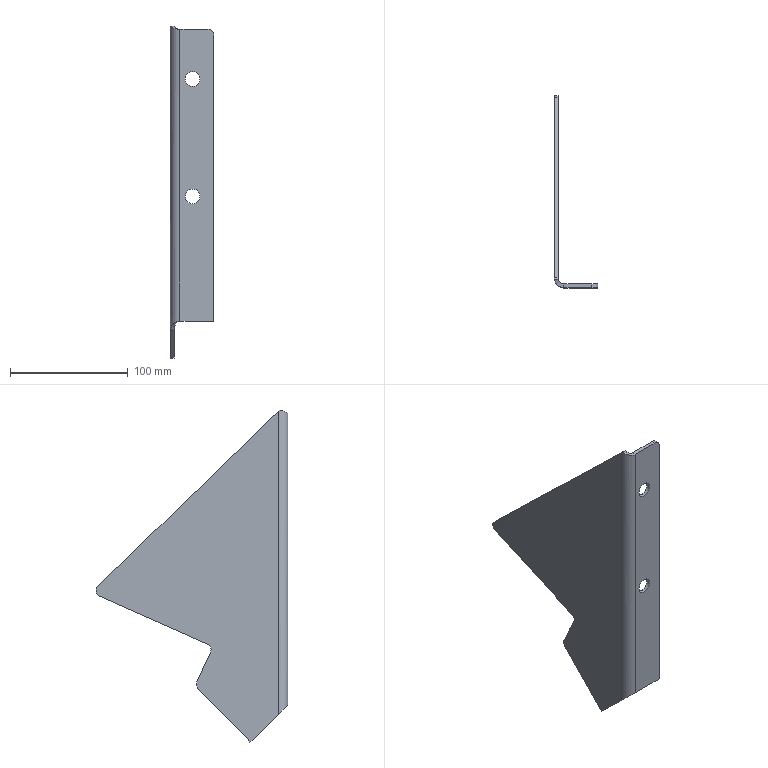Part | SolidWorks | features ICE 2, Fillet 1, FlatPattern 1, SMBaseFlange 1, SheetMetal 1 | 1 solid | 25 faces | box 37 x 163.164 x 282.329 mm | volume 98430 mm3 | plane 12 | cylinder 10 | spline 3 | commonest cylinder face diameters 10 x5 12.5 x4 16.4 x1
STEP:
#1=CARTESIAN_POINT('',(19.,3.2,-50.25));
#2=VERTEX_POINT('',#1);
#3=CARTESIAN_POINT('',(19.,3.2,-37.75));
#4=VERTEX_POINT('',#3);
#5=CARTESIAN_POINT('',(19.,3.2,-44.));
#6=DIRECTION('',(0.,1.,0.));
#7=DIRECTION('',(0.,0.,1.));
#8=AXIS2_PLACEMENT_3D('',#5,#6,#7);
#9=CIRCLE('',#8,6.25);
#10=EDGE_CURVE('',#2,#4,#9,.T.);
#11=ORIENTED_EDGE('',*,*,#10,.T.);
#12=CARTESIAN_POINT('',(19.,0.,-37.75));
#13=VERTEX_POINT('',#12);
#14=CARTESIAN_POINT('',(19.,163.164,-37.75));
#15=DIRECTION('',(0.,-1.,0.));
#16=VECTOR('',#15,1000.);
#17=LINE('',#14,#16);
#18=EDGE_CURVE('',#4,#13,#17,.T.);
#19=ORIENTED_EDGE('',*,*,#18,.T.);
#20=CARTESIAN_POINT('',(19.,0.,-50.25));
#21=VERTEX_POINT('',#20);
#22=CARTESIAN_POINT('',(19.,0.,-44.));
#23=DIRECTION('',(0.,-1.,0.));
#24=DIRECTION('',(0.,0.,-1.));
#25=AXIS2_PLACEMENT_3D('',#22,#23,#24);
#26=CIRCLE('',#25,6.25);
#27=EDGE_CURVE('',#13,#21,#26,.T.);
#28=ORIENTED_EDGE('',*,*,#27,.T.);
#29=CARTESIAN_POINT('',(19.,163.164,-50.25));
#30=DIRECTION('',(0.,-1.,0.));
#31=VECTOR('',#30,1000.);
#32=LINE('',#29,#31);
#33=EDGE_CURVE('',#2,#21,#32,.T.);
#34=ORIENTED_EDGE('',*,*,#33,.F.);
#35=EDGE_LOOP('',(#11,#19,#28,#34));
#36=FACE_OUTER_BOUND('',#35,.T.);
#37=CARTESIAN_POINT('',(19.,163.164,-44.));
#38=DIRECTION('',(0.,-1.,0.));
#39=DIRECTION('',(0.,0.,-1.));
#40=AXIS2_PLACEMENT_3D('',#37,#38,#39);
#41=CYLINDRICAL_SURFACE('',#40,6.25);
#42=ADVANCED_FACE('',(#36),#41,.F.);
#43=CARTESIAN_POINT('',(19.,3.2,49.75));
#44=VERTEX_POINT('',#43);
#45=CARTESIAN_POINT('',(19.,3.2,62.25));
#46=VERTEX_POINT('',#45);
#47=CARTESIAN_POINT('',(19.,3.2,56.));
#48=DIRECTION('',(0.,1.,0.));
#49=DIRECTION('',(0.,0.,1.));
#50=AXIS2_PLACEMENT_3D('',#47,#48,#49);
#51=CIRCLE('',#50,6.25);
#52=EDGE_CURVE('',#44,#46,#51,.T.);
#53=ORIENTED_EDGE('',*,*,#52,.T.);
#54=CARTESIAN_POINT('',(19.,0.,62.25));
#55=VERTEX_POINT('',#54);
#56=CARTESIAN_POINT('',(19.,163.164,62.25));
#57=DIRECTION('',(0.,-1.,0.));
#58=VECTOR('',#57,1000.);
#59=LINE('',#56,#58);
#60=EDGE_CURVE('',#46,#55,#59,.T.);
#61=ORIENTED_EDGE('',*,*,#60,.T.);
#62=CARTESIAN_POINT('',(19.,0.,49.75));
#63=VERTEX_POINT('',#62);
#64=CARTESIAN_POINT('',(19.,0.,56.));
#65=DIRECTION('',(0.,-1.,0.));
#66=DIRECTION('',(0.,0.,-1.));
#67=AXIS2_PLACEMENT_3D('',#64,#65,#66);
#68=CIRCLE('',#67,6.25);
#69=EDGE_CURVE('',#55,#63,#68,.T.);
#70=ORIENTED_EDGE('',*,*,#69,.T.);
#71=CARTESIAN_POINT('',(19.,163.164,49.75));
#72=DIRECTION('',(0.,-1.,0.));
#73=VECTOR('',#72,1000.);
#74=LINE('',#71,#73);
#75=EDGE_CURVE('',#44,#63,#74,.T.);
#76=ORIENTED_EDGE('',*,*,#75,.F.);
#77=EDGE_LOOP('',(#53,#61,#70,#76));
#78=FACE_OUTER_BOUND('',#77,.T.);
#79=CARTESIAN_POINT('',(19.,163.164,56.));
#80=DIRECTION('',(0.,-1.,0.));
#81=DIRECTION('',(0.,0.,-1.));
#82=AXIS2_PLACEMENT_3D('',#79,#80,#81);
#83=CYLINDRICAL_SURFACE('',#82,6.25);
#84=ADVANCED_FACE('',(#78),#83,.F.);
#85=CARTESIAN_POINT('',(19.,0.,-44.));
#86=DIRECTION('',(0.,-1.,0.));
#87=DIRECTION('',(0.,0.,-1.));
#88=AXIS2_PLACEMENT_3D('',#85,#86,#87);
#89=CIRCLE('',#88,6.25);
#90=EDGE_CURVE('',#21,#13,#89,.T.);
#91=ORIENTED_EDGE('',*,*,#90,.F.);
#92=ORIENTED_EDGE('',*,*,#27,.F.);
#93=EDGE_LOOP('',(#91,#92));
#94=FACE_BOUND('',#93,.T.);
#95=CARTESIAN_POINT('',(19.,0.,56.));
#96=DIRECTION('',(0.,-1.,0.));
#97=DIRECTION('',(0.,0.,-1.));
#98=AXIS2_PLACEMENT_3D('',#95,#96,#97);
#99=CIRCLE('',#98,6.25);
#100=EDGE_CURVE('',#63,#55,#99,.T.);
#101=ORIENTED_EDGE('',*,*,#100,.F.);
#102=ORIENTED_EDGE('',*,*,#69,.F.);
#103=EDGE_LOOP('',(#101,#102));
#104=FACE_BOUND('',#103,.T.);
#105=CARTESIAN_POINT('',(37.,0.,93.22));
#106=VERTEX_POINT('',#105);
#107=CARTESIAN_POINT('',(37.,0.,-150.));
#108=VERTEX_POINT('',#107);
#109=CARTESIAN_POINT('',(37.,0.,250.));
#110=DIRECTION('',(0.,0.,-1.));
#111=VECTOR('',#110,1000.);
#112=LINE('',#109,#111);
#113=EDGE_CURVE('',#106,#108,#112,.T.);
#114=ORIENTED_EDGE('',*,*,#113,.F.);
#115=CARTESIAN_POINT('',(32.,0.,98.22));
#116=VERTEX_POINT('',#115);
#117=CARTESIAN_POINT('',(32.,0.,93.22));
#118=DIRECTION('',(0.,-1.,0.));
#119=DIRECTION('',(0.,0.,1.));
#120=AXIS2_PLACEMENT_3D('',#117,#118,#119);
#121=CIRCLE('',#120,5.);
#122=EDGE_CURVE('',#106,#116,#121,.T.);
#123=ORIENTED_EDGE('',*,*,#122,.T.);
#124=CARTESIAN_POINT('',(8.2,0.,98.22));
#125=VERTEX_POINT('',#124);
#126=CARTESIAN_POINT('',(37.,0.,98.22));
#127=DIRECTION('',(-1.,0.,0.));
#128=VECTOR('',#127,1000.);
#129=LINE('',#126,#128);
#130=EDGE_CURVE('',#116,#125,#129,.T.);
#131=ORIENTED_EDGE('',*,*,#130,.T.);
#132=CARTESIAN_POINT('',(8.2,0.,-150.));
#133=VERTEX_POINT('',#132);
#134=CARTESIAN_POINT('',(8.2,0.,250.));
#135=DIRECTION('',(0.,0.,-1.));
#136=VECTOR('',#135,1000.);
#137=LINE('',#134,#136);
#138=EDGE_CURVE('',#125,#133,#137,.T.);
#139=ORIENTED_EDGE('',*,*,#138,.T.);
#140=CARTESIAN_POINT('',(37.,0.,-150.));
#141=DIRECTION('',(-1.,0.,0.));
#142=VECTOR('',#141,1000.);
#143=LINE('',#140,#142);
#144=EDGE_CURVE('',#108,#133,#143,.T.);
#145=ORIENTED_EDGE('',*,*,#144,.F.);
#146=EDGE_LOOP('',(#114,#123,#131,#139,#145));
#147=FACE_OUTER_BOUND('',#146,.T.);
#148=CARTESIAN_POINT('',(0.,0.,250.));
#149=DIRECTION('',(0.,1.,0.));
#150=DIRECTION('',(0.,0.,1.));
#151=AXIS2_PLACEMENT_3D('',#148,#149,#150);
#152=PLANE('',#151);
#153=ADVANCED_FACE('',(#94,#104,#147),#152,.F.);
#154=CARTESIAN_POINT('',(37.,3.2,93.22));
#155=VERTEX_POINT('',#154);
#156=CARTESIAN_POINT('',(37.,3.2,-150.));
#157=VERTEX_POINT('',#156);
#158=CARTESIAN_POINT('',(37.,3.2,250.));
#159=DIRECTION('',(0.,0.,-1.));
#160=VECTOR('',#159,1000.);
#161=LINE('',#158,#160);
#162=EDGE_CURVE('',#155,#157,#161,.T.);
#163=ORIENTED_EDGE('',*,*,#162,.F.);
#164=CARTESIAN_POINT('',(37.,3.2,93.22));
#165=DIRECTION('',(0.,-1.,0.));
#166=VECTOR('',#165,1000.);
#167=LINE('',#164,#166);
#168=EDGE_CURVE('',#155,#106,#167,.T.);
#169=ORIENTED_EDGE('',*,*,#168,.T.);
#170=ORIENTED_EDGE('',*,*,#113,.T.);
#171=CARTESIAN_POINT('',(37.,0.,-150.));
#172=DIRECTION('',(0.,1.,0.));
#173=VECTOR('',#172,1000.);
#174=LINE('',#171,#173);
#175=EDGE_CURVE('',#108,#157,#174,.T.);
#176=ORIENTED_EDGE('',*,*,#175,.T.);
#177=EDGE_LOOP('',(#163,#169,#170,#176));
#178=FACE_OUTER_BOUND('',#177,.T.);
#179=CARTESIAN_POINT('',(37.,3.2,250.));
#180=DIRECTION('',(1.,0.,0.));
#181=DIRECTION('',(0.,0.,-1.));
#182=AXIS2_PLACEMENT_3D('',#179,#180,#181);
#183=PLANE('',#182);
#184=ADVANCED_FACE('',(#178),#183,.T.);
#185=ORIENTED_EDGE('',*,*,#10,.F.);
#186=CARTESIAN_POINT('',(19.,3.2,-44.));
#187=DIRECTION('',(0.,1.,0.));
#188=DIRECTION('',(0.,0.,1.));
#189=AXIS2_PLACEMENT_3D('',#186,#187,#188);
#190=CIRCLE('',#189,6.25);
#191=EDGE_CURVE('',#4,#2,#190,.T.);
#192=ORIENTED_EDGE('',*,*,#191,.F.);
#193=EDGE_LOOP('',(#185,#192));
#194=FACE_BOUND('',#193,.T.);
#195=ORIENTED_EDGE('',*,*,#52,.F.);
#196=CARTESIAN_POINT('',(19.,3.2,56.));
#197=DIRECTION('',(0.,1.,0.));
#198=DIRECTION('',(0.,0.,1.));
#199=AXIS2_PLACEMENT_3D('',#196,#197,#198);
#200=CIRCLE('',#199,6.25);
#201=EDGE_CURVE('',#46,#44,#200,.T.);
#202=ORIENTED_EDGE('',*,*,#201,.F.);
#203=EDGE_LOOP('',(#195,#202));
#204=FACE_BOUND('',#203,.T.);
#205=CARTESIAN_POINT('',(32.,3.2,98.22));
#206=VERTEX_POINT('',#205);
#207=CARTESIAN_POINT('',(8.2,3.2,98.22));
#208=VERTEX_POINT('',#207);
#209=CARTESIAN_POINT('',(0.,3.2,98.22));
#210=DIRECTION('',(-1.,0.,0.));
#211=VECTOR('',#210,1000.);
#212=LINE('',#209,#211);
#213=EDGE_CURVE('',#206,#208,#212,.T.);
#214=ORIENTED_EDGE('',*,*,#213,.F.);
#215=CARTESIAN_POINT('',(32.,3.2,93.22));
#216=DIRECTION('',(0.,1.,0.));
#217=DIRECTION('',(0.,0.,1.));
#218=AXIS2_PLACEMENT_3D('',#215,#216,#217);
#219=CIRCLE('',#218,5.);
#220=EDGE_CURVE('',#206,#155,#219,.T.);
#221=ORIENTED_EDGE('',*,*,#220,.T.);
#222=ORIENTED_EDGE('',*,*,#162,.T.);
#223=CARTESIAN_POINT('',(8.2,3.2,-150.));
#224=VERTEX_POINT('',#223);
#225=CARTESIAN_POINT('',(0.,3.2,-150.));
#226=DIRECTION('',(-1.,0.,0.));
#227=VECTOR('',#226,1000.);
#228=LINE('',#225,#227);
#229=EDGE_CURVE('',#157,#224,#228,.T.);
#230=ORIENTED_EDGE('',*,*,#229,.T.);
#231=CARTESIAN_POINT('',(8.2,3.2,250.));
#232=DIRECTION('',(0.,0.,-1.));
#233=VECTOR('',#232,1000.);
#234=LINE('',#231,#233);
#235=EDGE_CURVE('',#208,#224,#234,.T.);
#236=ORIENTED_EDGE('',*,*,#235,.F.);
#237=EDGE_LOOP('',(#214,#221,#222,#230,#236));
#238=FACE_OUTER_BOUND('',#237,.T.);
#239=CARTESIAN_POINT('',(0.,3.2,250.));
#240=DIRECTION('',(0.,1.,0.));
#241=DIRECTION('',(0.,0.,1.));
#242=AXIS2_PLACEMENT_3D('',#239,#240,#241);
#243=PLANE('',#242);
#244=ADVANCED_FACE('',(#194,#204,#238),#243,.T.);
#245=ORIENTED_EDGE('',*,*,#235,.T.);
#246=CARTESIAN_POINT('',(3.2,8.2,-157.97));
#247=VERTEX_POINT('',#246);
#248=CARTESIAN_POINT('',(3.2,8.2,-157.97));
#249=CARTESIAN_POINT('',(3.2,5.271,-153.301));
#250=CARTESIAN_POINT('',(5.271,3.2,-150.));
#251=CARTESIAN_POINT('',(8.2,3.2,-150.));
#252=(BOUNDED_CURVE()B_SPLINE_CURVE(3,(#248,#249,#250,#251),.UNSPECIFIED.,.F.,.F.)B_SPLINE_CURVE_WITH_KNOTS((4,4),(1.571,3.142),.UNSPECIFIED.)CURVE()GEOMETRIC_REPRESENTATION_ITEM()RATIONAL_B_SPLINE_CURVE((1.,0.8047,0.8047,1.))REPRESENTATION_ITEM(''));
#253=EDGE_CURVE('',#247,#224,#252,.T.);
#254=ORIENTED_EDGE('',*,*,#253,.F.);
#255=CARTESIAN_POINT('',(3.2,8.2,100.011));
#256=VERTEX_POINT('',#255);
#257=CARTESIAN_POINT('',(3.2,8.2,250.));
#258=DIRECTION('',(0.,0.,-1.));
#259=VECTOR('',#258,1000.);
#260=LINE('',#257,#259);
#261=EDGE_CURVE('',#256,#247,#260,.T.);
#262=ORIENTED_EDGE('',*,*,#261,.F.);
#263=CARTESIAN_POINT('',(3.297,7.219,100.965));
#264=VERTEX_POINT('',#263);
#265=CARTESIAN_POINT('',(3.297,7.219,100.965));
#266=CARTESIAN_POINT('',(3.233,7.542,100.651));
#267=CARTESIAN_POINT('',(3.2,7.87,100.332));
#268=CARTESIAN_POINT('',(3.2,8.2,100.011));
#269=(BOUNDED_CURVE()B_SPLINE_CURVE(3,(#265,#266,#267,#268),.UNSPECIFIED.,.F.,.F.)B_SPLINE_CURVE_WITH_KNOTS((4,4),(4.515,4.712),.UNSPECIFIED.)CURVE()GEOMETRIC_REPRESENTATION_ITEM()RATIONAL_B_SPLINE_CURVE((1.,0.9967,0.9967,1.))REPRESENTATION_ITEM(''));
#270=EDGE_CURVE('',#264,#256,#269,.T.);
#271=ORIENTED_EDGE('',*,*,#270,.F.);
#272=CARTESIAN_POINT('',(8.2,3.2,98.22));
#273=CARTESIAN_POINT('',(5.711,3.2,98.22));
#274=CARTESIAN_POINT('',(3.786,4.778,99.298));
#275=CARTESIAN_POINT('',(3.297,7.219,100.965));
#276=(BOUNDED_CURVE()B_SPLINE_CURVE(3,(#272,#273,#274,#275),.UNSPECIFIED.,.F.,.T.)B_SPLINE_CURVE_WITH_KNOTS((4,4),(0.,1.373),.UNSPECIFIED.)CURVE()GEOMETRIC_REPRESENTATION_ITEM()RATIONAL_B_SPLINE_CURVE((1.,0.8489,0.8489,1.))REPRESENTATION_ITEM(''));
#277=EDGE_CURVE('',#208,#264,#276,.T.);
#278=ORIENTED_EDGE('',*,*,#277,.F.);
#279=EDGE_LOOP('',(#245,#254,#262,#271,#278));
#280=FACE_OUTER_BOUND('',#279,.T.);
#281=CARTESIAN_POINT('',(8.2,8.2,250.));
#282=DIRECTION('',(0.,0.,-1.));
#283=DIRECTION('',(-1.,0.,0.));
#284=AXIS2_PLACEMENT_3D('',#281,#282,#283);
#285=CYLINDRICAL_SURFACE('',#284,5.);
#286=ADVANCED_FACE('',(#280),#285,.F.);
#287=CARTESIAN_POINT('',(3.2,32.27,-181.363));
#288=VERTEX_POINT('',#287);
#289=CARTESIAN_POINT('',(3.2,76.568,-135.785));
#290=VERTEX_POINT('',#289);
#291=CARTESIAN_POINT('',(3.2,32.27,-181.363));
#292=DIRECTION('',(0.,0.697,0.7171));
#293=VECTOR('',#292,1000.);
#294=LINE('',#291,#293);
#295=EDGE_CURVE('',#288,#290,#294,.T.);
#296=ORIENTED_EDGE('',*,*,#295,.T.);
#297=CARTESIAN_POINT('',(3.2,77.518,-130.196));
#298=VERTEX_POINT('',#297);
#299=CARTESIAN_POINT('',(3.2,72.982,-132.3));
#300=DIRECTION('',(1.,0.,0.));
#301=DIRECTION('',(0.,0.,-1.));
#302=AXIS2_PLACEMENT_3D('',#299,#300,#301);
#303=CIRCLE('',#302,5.);
#304=EDGE_CURVE('',#290,#298,#303,.T.);
#305=ORIENTED_EDGE('',*,*,#304,.T.);
#306=CARTESIAN_POINT('',(3.2,65.782,-104.904));
#307=VERTEX_POINT('',#306);
#308=CARTESIAN_POINT('',(3.2,78.966,-133.317));
#309=DIRECTION('',(0.,-0.4209,0.9071));
#310=VECTOR('',#309,1000.);
#311=LINE('',#308,#310);
#312=EDGE_CURVE('',#298,#307,#311,.T.);
#313=ORIENTED_EDGE('',*,*,#312,.T.);
#314=CARTESIAN_POINT('',(3.2,68.283,-98.232));
#315=VERTEX_POINT('',#314);
#316=CARTESIAN_POINT('',(3.2,70.318,-102.799));
#317=DIRECTION('',(-1.,0.,0.));
#318=DIRECTION('',(0.,0.,-1.));
#319=AXIS2_PLACEMENT_3D('',#316,#317,#318);
#320=CIRCLE('',#319,5.);
#321=EDGE_CURVE('',#307,#315,#320,.T.);
#322=ORIENTED_EDGE('',*,*,#321,.T.);
#323=CARTESIAN_POINT('',(3.2,160.199,-57.28));
#324=VERTEX_POINT('',#323);
#325=CARTESIAN_POINT('',(3.2,63.645,-100.298));
#326=DIRECTION('',(0.,0.9134,0.407));
#327=VECTOR('',#326,1000.);
#328=LINE('',#325,#327);
#329=EDGE_CURVE('',#315,#324,#328,.T.);
#330=ORIENTED_EDGE('',*,*,#329,.T.);
#331=CARTESIAN_POINT('',(3.2,161.649,-49.127));
#332=VERTEX_POINT('',#331);
#333=CARTESIAN_POINT('',(3.2,158.164,-52.713));
#334=DIRECTION('',(1.,0.,0.));
#335=DIRECTION('',(0.,0.,-1.));
#336=AXIS2_PLACEMENT_3D('',#333,#334,#335);
#337=CIRCLE('',#336,5.);
#338=EDGE_CURVE('',#324,#332,#337,.T.);
#339=ORIENTED_EDGE('',*,*,#338,.T.);
#340=CARTESIAN_POINT('',(3.2,166.945,-54.274));
#341=DIRECTION('',(0.,-0.7171,0.697));
#342=VECTOR('',#341,1000.);
#343=LINE('',#340,#342);
#344=EDGE_CURVE('',#332,#256,#343,.T.);
#345=ORIENTED_EDGE('',*,*,#344,.T.);
#346=ORIENTED_EDGE('',*,*,#261,.T.);
#347=CARTESIAN_POINT('',(3.2,32.27,-181.363));
#348=DIRECTION('',(0.,0.7171,-0.697));
#349=VECTOR('',#348,1000.);
#350=LINE('',#347,#349);
#351=EDGE_CURVE('',#247,#288,#350,.T.);
#352=ORIENTED_EDGE('',*,*,#351,.T.);
#353=EDGE_LOOP('',(#296,#305,#313,#322,#330,#339,#345,#346,#352));
#354=FACE_OUTER_BOUND('',#353,.T.);
#355=CARTESIAN_POINT('',(3.2,0.,250.));
#356=DIRECTION('',(1.,0.,0.));
#357=DIRECTION('',(0.,0.,-1.));
#358=AXIS2_PLACEMENT_3D('',#355,#356,#357);
#359=PLANE('',#358);
#360=ADVANCED_FACE('',(#354),#359,.T.);
#361=CARTESIAN_POINT('',(0.,77.518,-130.196));
#362=VERTEX_POINT('',#361);
#363=CARTESIAN_POINT('',(0.,65.782,-104.904));
#364=VERTEX_POINT('',#363);
#365=CARTESIAN_POINT('',(0.,78.966,-133.317));
#366=DIRECTION('',(0.,-0.4209,0.9071));
#367=VECTOR('',#366,1000.);
#368=LINE('',#365,#367);
#369=EDGE_CURVE('',#362,#364,#368,.T.);
#370=ORIENTED_EDGE('',*,*,#369,.F.);
#371=CARTESIAN_POINT('',(0.,76.568,-135.785));
#372=VERTEX_POINT('',#371);
#373=CARTESIAN_POINT('',(0.,72.982,-132.3));
#374=DIRECTION('',(-1.,0.,0.));
#375=DIRECTION('',(0.,0.,-1.));
#376=AXIS2_PLACEMENT_3D('',#373,#374,#375);
#377=CIRCLE('',#376,5.);
#378=EDGE_CURVE('',#362,#372,#377,.T.);
#379=ORIENTED_EDGE('',*,*,#378,.T.);
#380=CARTESIAN_POINT('',(0.,32.27,-181.363));
#381=VERTEX_POINT('',#380);
#382=CARTESIAN_POINT('',(0.,32.27,-181.363));
#383=DIRECTION('',(0.,0.697,0.7171));
#384=VECTOR('',#383,1000.);
#385=LINE('',#382,#384);
#386=EDGE_CURVE('',#381,#372,#385,.T.);
#387=ORIENTED_EDGE('',*,*,#386,.F.);
#388=CARTESIAN_POINT('',(0.,8.2,-157.97));
#389=VERTEX_POINT('',#388);
#390=CARTESIAN_POINT('',(0.,32.27,-181.363));
#391=DIRECTION('',(0.,0.7171,-0.697));
#392=VECTOR('',#391,1000.);
#393=LINE('',#390,#392);
#394=EDGE_CURVE('',#389,#381,#393,.T.);
#395=ORIENTED_EDGE('',*,*,#394,.F.);
#396=CARTESIAN_POINT('',(0.,8.2,100.011));
#397=VERTEX_POINT('',#396);
#398=CARTESIAN_POINT('',(0.,8.2,250.));
#399=DIRECTION('',(0.,0.,-1.));
#400=VECTOR('',#399,1000.);
#401=LINE('',#398,#400);
#402=EDGE_CURVE('',#397,#389,#401,.T.);
#403=ORIENTED_EDGE('',*,*,#402,.F.);
#404=CARTESIAN_POINT('',(0.,161.649,-49.127));
#405=VERTEX_POINT('',#404);
#406=CARTESIAN_POINT('',(0.,166.945,-54.274));
#407=DIRECTION('',(0.,-0.7171,0.697));
#408=VECTOR('',#407,1000.);
#409=LINE('',#406,#408);
#410=EDGE_CURVE('',#405,#397,#409,.T.);
#411=ORIENTED_EDGE('',*,*,#410,.F.);
#412=CARTESIAN_POINT('',(0.,160.199,-57.28));
#413=VERTEX_POINT('',#412);
#414=CARTESIAN_POINT('',(0.,158.164,-52.713));
#415=DIRECTION('',(-1.,0.,0.));
#416=DIRECTION('',(0.,0.,-1.));
#417=AXIS2_PLACEMENT_3D('',#414,#415,#416);
#418=CIRCLE('',#417,5.);
#419=EDGE_CURVE('',#405,#413,#418,.T.);
#420=ORIENTED_EDGE('',*,*,#419,.T.);
#421=CARTESIAN_POINT('',(0.,68.283,-98.232));
#422=VERTEX_POINT('',#421);
#423=CARTESIAN_POINT('',(0.,63.645,-100.298));
#424=DIRECTION('',(0.,0.9134,0.407));
#425=VECTOR('',#424,1000.);
#426=LINE('',#423,#425);
#427=EDGE_CURVE('',#422,#413,#426,.T.);
#428=ORIENTED_EDGE('',*,*,#427,.F.);
#429=CARTESIAN_POINT('',(0.,70.318,-102.799));
#430=DIRECTION('',(1.,0.,0.));
#431=DIRECTION('',(0.,0.,-1.));
#432=AXIS2_PLACEMENT_3D('',#429,#430,#431);
#433=CIRCLE('',#432,5.);
#434=EDGE_CURVE('',#422,#364,#433,.T.);
#435=ORIENTED_EDGE('',*,*,#434,.T.);
#436=EDGE_LOOP('',(#370,#379,#387,#395,#403,#411,#420,#428,#435));
#437=FACE_OUTER_BOUND('',#436,.T.);
#438=CARTESIAN_POINT('',(0.,0.,250.));
#439=DIRECTION('',(1.,0.,0.));
#440=DIRECTION('',(0.,0.,-1.));
#441=AXIS2_PLACEMENT_3D('',#438,#439,#440);
#442=PLANE('',#441);
#443=ADVANCED_FACE('',(#437),#442,.F.);
#444=CARTESIAN_POINT('',(0.,8.2,-157.97));
#445=CARTESIAN_POINT('',(0.,3.397,-153.301));
#446=CARTESIAN_POINT('',(3.397,0.,-150.));
#447=CARTESIAN_POINT('',(8.2,0.,-150.));
#448=(BOUNDED_CURVE()B_SPLINE_CURVE(3,(#444,#445,#446,#447),.UNSPECIFIED.,.F.,.F.)B_SPLINE_CURVE_WITH_KNOTS((4,4),(1.571,3.142),.UNSPECIFIED.)CURVE()GEOMETRIC_REPRESENTATION_ITEM()RATIONAL_B_SPLINE_CURVE((1.,0.8047,0.8047,1.))REPRESENTATION_ITEM(''));
#449=EDGE_CURVE('',#389,#133,#448,.T.);
#450=ORIENTED_EDGE('',*,*,#449,.T.);
#451=ORIENTED_EDGE('',*,*,#138,.F.);
#452=CARTESIAN_POINT('',(0.1595,6.59,100.965));
#453=VERTEX_POINT('',#452);
#454=CARTESIAN_POINT('',(8.2,0.,98.22));
#455=CARTESIAN_POINT('',(4.118,0.,98.22));
#456=CARTESIAN_POINT('',(0.9608,2.588,99.298));
#457=CARTESIAN_POINT('',(0.1595,6.59,100.965));
#458=(BOUNDED_CURVE()B_SPLINE_CURVE(3,(#454,#455,#456,#457),.UNSPECIFIED.,.F.,.F.)B_SPLINE_CURVE_WITH_KNOTS((4,4),(0.,1.373),.UNSPECIFIED.)CURVE()GEOMETRIC_REPRESENTATION_ITEM()RATIONAL_B_SPLINE_CURVE((1.,0.8489,0.8489,1.))REPRESENTATION_ITEM(''));
#459=EDGE_CURVE('',#125,#453,#458,.T.);
#460=ORIENTED_EDGE('',*,*,#459,.T.);
#461=CARTESIAN_POINT('',(0.1595,6.59,100.965));
#462=CARTESIAN_POINT('',(0.05335,7.121,100.651));
#463=CARTESIAN_POINT('',(0.,7.659,100.332));
#464=CARTESIAN_POINT('',(0.,8.2,100.011));
#465=(BOUNDED_CURVE()B_SPLINE_CURVE(3,(#461,#462,#463,#464),.UNSPECIFIED.,.F.,.F.)B_SPLINE_CURVE_WITH_KNOTS((4,4),(4.515,4.712),.UNSPECIFIED.)CURVE()GEOMETRIC_REPRESENTATION_ITEM()RATIONAL_B_SPLINE_CURVE((1.,0.9967,0.9967,1.))REPRESENTATION_ITEM(''));
#466=EDGE_CURVE('',#453,#397,#465,.T.);
#467=ORIENTED_EDGE('',*,*,#466,.T.);
#468=ORIENTED_EDGE('',*,*,#402,.T.);
#469=EDGE_LOOP('',(#450,#451,#460,#467,#468));
#470=FACE_OUTER_BOUND('',#469,.T.);
#471=CARTESIAN_POINT('',(8.2,8.2,250.));
#472=DIRECTION('',(0.,0.,-1.));
#473=DIRECTION('',(-1.,0.,0.));
#474=AXIS2_PLACEMENT_3D('',#471,#472,#473);
#475=CYLINDRICAL_SURFACE('',#474,8.2);
#476=ADVANCED_FACE('',(#470),#475,.T.);
#477=ORIENTED_EDGE('',*,*,#130,.F.);
#478=CARTESIAN_POINT('',(32.,0.,98.22));
#479=DIRECTION('',(0.,1.,0.));
#480=VECTOR('',#479,1000.);
#481=LINE('',#478,#480);
#482=EDGE_CURVE('',#116,#206,#481,.T.);
#483=ORIENTED_EDGE('',*,*,#482,.T.);
#484=ORIENTED_EDGE('',*,*,#213,.T.);
#485=CARTESIAN_POINT('',(8.2,0.,98.22));
#486=DIRECTION('',(0.,1.,0.));
#487=VECTOR('',#486,1000.);
#488=LINE('',#485,#487);
#489=EDGE_CURVE('',#125,#208,#488,.T.);
#490=ORIENTED_EDGE('',*,*,#489,.F.);
#491=EDGE_LOOP('',(#477,#483,#484,#490));
#492=FACE_OUTER_BOUND('',#491,.T.);
#493=CARTESIAN_POINT('',(37.,0.,98.22));
#494=DIRECTION('',(0.,0.,-1.));
#495=DIRECTION('',(-1.,0.,0.));
#496=AXIS2_PLACEMENT_3D('',#493,#494,#495);
#497=PLANE('',#496);
#498=ADVANCED_FACE('',(#492),#497,.F.);
#499=CARTESIAN_POINT('',(0.,8.2,-157.97));
#500=DIRECTION('',(1.,0.,0.));
#501=VECTOR('',#500,1000.);
#502=LINE('',#499,#501);
#503=EDGE_CURVE('',#389,#247,#502,.T.);
#504=ORIENTED_EDGE('',*,*,#503,.F.);
#505=ORIENTED_EDGE('',*,*,#394,.T.);
#506=CARTESIAN_POINT('',(0.,32.27,-181.363));
#507=DIRECTION('',(1.,0.,0.));
#508=VECTOR('',#507,1000.);
#509=LINE('',#506,#508);
#510=EDGE_CURVE('',#381,#288,#509,.T.);
#511=ORIENTED_EDGE('',*,*,#510,.T.);
#512=ORIENTED_EDGE('',*,*,#351,.F.);
#513=EDGE_LOOP('',(#504,#505,#511,#512));
#514=FACE_OUTER_BOUND('',#513,.T.);
#515=CARTESIAN_POINT('',(0.,32.27,-181.363));
#516=DIRECTION('',(0.,-0.697,-0.7171));
#517=DIRECTION('',(0.,0.7171,-0.697));
#518=AXIS2_PLACEMENT_3D('',#515,#516,#517);
#519=PLANE('',#518);
#520=ADVANCED_FACE('',(#514),#519,.T.);
#521=ORIENTED_EDGE('',*,*,#386,.T.);
#522=CARTESIAN_POINT('',(0.,76.568,-135.785));
#523=DIRECTION('',(1.,0.,0.));
#524=VECTOR('',#523,1000.);
#525=LINE('',#522,#524);
#526=EDGE_CURVE('',#372,#290,#525,.T.);
#527=ORIENTED_EDGE('',*,*,#526,.T.);
#528=ORIENTED_EDGE('',*,*,#295,.F.);
#529=ORIENTED_EDGE('',*,*,#510,.F.);
#530=EDGE_LOOP('',(#521,#527,#528,#529));
#531=FACE_OUTER_BOUND('',#530,.T.);
#532=CARTESIAN_POINT('',(0.,32.27,-181.363));
#533=DIRECTION('',(0.,0.7171,-0.697));
#534=DIRECTION('',(0.,0.697,0.7171));
#535=AXIS2_PLACEMENT_3D('',#532,#533,#534);
#536=PLANE('',#535);
#537=ADVANCED_FACE('',(#531),#536,.T.);
#538=ORIENTED_EDGE('',*,*,#312,.F.);
#539=CARTESIAN_POINT('',(0.,77.518,-130.196));
#540=DIRECTION('',(-1.,0.,0.));
#541=VECTOR('',#540,1000.);
#542=LINE('',#539,#541);
#543=EDGE_CURVE('',#298,#362,#542,.T.);
#544=ORIENTED_EDGE('',*,*,#543,.T.);
#545=ORIENTED_EDGE('',*,*,#369,.T.);
#546=CARTESIAN_POINT('',(3.2,65.782,-104.904));
#547=DIRECTION('',(1.,0.,0.));
#548=VECTOR('',#547,1000.);
#549=LINE('',#546,#548);
#550=EDGE_CURVE('',#364,#307,#549,.T.);
#551=ORIENTED_EDGE('',*,*,#550,.T.);
#552=EDGE_LOOP('',(#538,#544,#545,#551));
#553=FACE_OUTER_BOUND('',#552,.T.);
#554=CARTESIAN_POINT('',(0.,78.966,-133.317));
#555=DIRECTION('',(0.,0.9071,0.4209));
#556=DIRECTION('',(0.,-0.4209,0.9071));
#557=AXIS2_PLACEMENT_3D('',#554,#555,#556);
#558=PLANE('',#557);
#559=ADVANCED_FACE('',(#553),#558,.T.);
#560=ORIENTED_EDGE('',*,*,#329,.F.);
#561=CARTESIAN_POINT('',(0.,68.283,-98.232));
#562=DIRECTION('',(-1.,0.,0.));
#563=VECTOR('',#562,1000.);
#564=LINE('',#561,#563);
#565=EDGE_CURVE('',#315,#422,#564,.T.);
#566=ORIENTED_EDGE('',*,*,#565,.T.);
#567=ORIENTED_EDGE('',*,*,#427,.T.);
#568=CARTESIAN_POINT('',(0.,160.199,-57.28));
#569=DIRECTION('',(1.,0.,0.));
#570=VECTOR('',#569,1000.);
#571=LINE('',#568,#570);
#572=EDGE_CURVE('',#413,#324,#571,.T.);
#573=ORIENTED_EDGE('',*,*,#572,.T.);
#574=EDGE_LOOP('',(#560,#566,#567,#573));
#575=FACE_OUTER_BOUND('',#574,.T.);
#576=CARTESIAN_POINT('',(0.,63.645,-100.298));
#577=DIRECTION('',(0.,0.407,-0.9134));
#578=DIRECTION('',(0.,0.9134,0.407));
#579=AXIS2_PLACEMENT_3D('',#576,#577,#578);
#580=PLANE('',#579);
#581=ADVANCED_FACE('',(#575),#580,.T.);
#582=ORIENTED_EDGE('',*,*,#344,.F.);
#583=CARTESIAN_POINT('',(0.,161.649,-49.127));
#584=DIRECTION('',(-1.,0.,0.));
#585=VECTOR('',#584,1000.);
#586=LINE('',#583,#585);
#587=EDGE_CURVE('',#332,#405,#586,.T.);
#588=ORIENTED_EDGE('',*,*,#587,.T.);
#589=ORIENTED_EDGE('',*,*,#410,.T.);
#590=CARTESIAN_POINT('',(0.,8.2,100.011));
#591=DIRECTION('',(1.,0.,0.));
#592=VECTOR('',#591,1000.);
#593=LINE('',#590,#592);
#594=EDGE_CURVE('',#397,#256,#593,.T.);
#595=ORIENTED_EDGE('',*,*,#594,.T.);
#596=EDGE_LOOP('',(#582,#588,#589,#595));
#597=FACE_OUTER_BOUND('',#596,.T.);
#598=CARTESIAN_POINT('',(0.,166.945,-54.274));
#599=DIRECTION('',(0.,0.697,0.7171));
#600=DIRECTION('',(0.,-0.7171,0.697));
#601=AXIS2_PLACEMENT_3D('',#598,#599,#600);
#602=PLANE('',#601);
#603=ADVANCED_FACE('',(#597),#602,.T.);
#604=CARTESIAN_POINT('',(8.2,0.,-150.));
#605=DIRECTION('',(0.,1.,0.));
#606=VECTOR('',#605,1000.);
#607=LINE('',#604,#606);
#608=EDGE_CURVE('',#133,#224,#607,.T.);
#609=ORIENTED_EDGE('',*,*,#608,.F.);
#610=ORIENTED_EDGE('',*,*,#449,.F.);
#611=ORIENTED_EDGE('',*,*,#503,.T.);
#612=ORIENTED_EDGE('',*,*,#253,.T.);
#613=EDGE_LOOP('',(#609,#610,#611,#612));
#614=FACE_OUTER_BOUND('',#613,.T.);
#615=CARTESIAN_POINT('',(8.2,13.2,-165.939));
#616=CARTESIAN_POINT('',(8.2,14.267,-165.939));
#617=CARTESIAN_POINT('',(8.2,15.333,-165.939));
#618=CARTESIAN_POINT('',(8.2,16.4,-165.939));
#619=CARTESIAN_POINT('',(-1.8,13.2,-165.939));
#620=CARTESIAN_POINT('',(-3.933,14.267,-165.939));
#621=CARTESIAN_POINT('',(-6.067,15.333,-165.939));
#622=CARTESIAN_POINT('',(-8.2,16.4,-165.939));
#623=CARTESIAN_POINT('',(-1.8,3.2,-150.));
#624=CARTESIAN_POINT('',(-3.933,2.133,-150.));
#625=CARTESIAN_POINT('',(-6.067,1.067,-150.));
#626=CARTESIAN_POINT('',(-8.2,0.,-150.));
#627=CARTESIAN_POINT('',(8.2,3.2,-150.));
#628=CARTESIAN_POINT('',(8.2,2.133,-150.));
#629=CARTESIAN_POINT('',(8.2,1.067,-150.));
#630=CARTESIAN_POINT('',(8.2,0.,-150.));
#631=CARTESIAN_POINT('',(18.2,3.2,-150.));
#632=CARTESIAN_POINT('',(20.333,2.133,-150.));
#633=CARTESIAN_POINT('',(22.467,1.067,-150.));
#634=CARTESIAN_POINT('',(24.6,0.,-150.));
#635=CARTESIAN_POINT('',(18.2,13.2,-165.939));
#636=CARTESIAN_POINT('',(20.333,14.267,-165.939));
#637=CARTESIAN_POINT('',(22.467,15.333,-165.939));
#638=CARTESIAN_POINT('',(24.6,16.4,-165.939));
#639=CARTESIAN_POINT('',(8.2,13.2,-165.939));
#640=CARTESIAN_POINT('',(8.2,14.267,-165.939));
#641=CARTESIAN_POINT('',(8.2,15.333,-165.939));
#642=CARTESIAN_POINT('',(8.2,16.4,-165.939));
#643=(BOUNDED_SURFACE()B_SPLINE_SURFACE(3,3,((#615,#616,#617,#618),(#619,#620,#621,#622),(#623,#624,#625,#626),(#627,#628,#629,#630),(#631,#632,#633,#634),(#635,#636,#637,#638),(#639,#640,#641,#642)),.UNSPECIFIED.,.T.,.F.,.F.)B_SPLINE_SURFACE_WITH_KNOTS((4,3,4),(4,4),(0.,0.5,1.),(0.,1.),.UNSPECIFIED.)GEOMETRIC_REPRESENTATION_ITEM()RATIONAL_B_SPLINE_SURFACE(((1.,1.,1.,1.),(0.3333,0.3333,0.3333,0.3333),(0.3333,0.3333,0.3333,0.3333),(1.,1.,1.,1.),(0.3333,0.3333,0.3333,0.3333),(0.3333,0.3333,0.3333,0.3333),(1.,1.,1.,1.)))REPRESENTATION_ITEM('')SURFACE());
#644=ADVANCED_FACE('',(#614),#643,.T.);
#645=ORIENTED_EDGE('',*,*,#175,.F.);
#646=ORIENTED_EDGE('',*,*,#144,.T.);
#647=ORIENTED_EDGE('',*,*,#608,.T.);
#648=ORIENTED_EDGE('',*,*,#229,.F.);
#649=EDGE_LOOP('',(#645,#646,#647,#648));
#650=FACE_OUTER_BOUND('',#649,.T.);
#651=CARTESIAN_POINT('',(37.,0.,-150.));
#652=DIRECTION('',(0.,0.,-1.));
#653=DIRECTION('',(-1.,0.,0.));
#654=AXIS2_PLACEMENT_3D('',#651,#652,#653);
#655=PLANE('',#654);
#656=ADVANCED_FACE('',(#650),#655,.T.);
#657=CARTESIAN_POINT('',(3.297,7.219,100.965));
#658=CARTESIAN_POINT('',(2.251,7.009,100.965));
#659=CARTESIAN_POINT('',(1.205,6.8,100.965));
#660=CARTESIAN_POINT('',(0.1595,6.59,100.965));
#661=(BOUNDED_CURVE()B_SPLINE_CURVE(3,(#657,#658,#659,#660),.UNSPECIFIED.,.F.,.F.)B_SPLINE_CURVE_WITH_KNOTS((4,4),(0.,0.0032),.UNSPECIFIED.)CURVE()GEOMETRIC_REPRESENTATION_ITEM()RATIONAL_B_SPLINE_CURVE((0.5049,0.5049,0.5049,0.5049))REPRESENTATION_ITEM(''));
#662=EDGE_CURVE('',#264,#453,#661,.T.);
#663=ORIENTED_EDGE('',*,*,#662,.T.);
#664=ORIENTED_EDGE('',*,*,#459,.F.);
#665=ORIENTED_EDGE('',*,*,#489,.T.);
#666=ORIENTED_EDGE('',*,*,#277,.T.);
#667=EDGE_LOOP('',(#663,#664,#665,#666));
#668=FACE_OUTER_BOUND('',#667,.T.);
#669=CARTESIAN_POINT('',(8.2,3.2,98.22));
#670=CARTESIAN_POINT('',(8.2,2.133,98.22));
#671=CARTESIAN_POINT('',(8.2,1.067,98.22));
#672=CARTESIAN_POINT('',(8.2,0.,98.22));
#673=CARTESIAN_POINT('',(-1.8,3.2,98.22));
#674=CARTESIAN_POINT('',(-3.933,2.133,98.22));
#675=CARTESIAN_POINT('',(-6.067,1.067,98.22));
#676=CARTESIAN_POINT('',(-8.2,0.,98.22));
#677=CARTESIAN_POINT('',(-1.8,13.2,105.052));
#678=CARTESIAN_POINT('',(-3.933,14.267,105.052));
#679=CARTESIAN_POINT('',(-6.067,15.333,105.052));
#680=CARTESIAN_POINT('',(-8.2,16.4,105.052));
#681=CARTESIAN_POINT('',(8.2,13.2,105.052));
#682=CARTESIAN_POINT('',(8.2,14.267,105.052));
#683=CARTESIAN_POINT('',(8.2,15.333,105.052));
#684=CARTESIAN_POINT('',(8.2,16.4,105.052));
#685=CARTESIAN_POINT('',(18.2,13.2,105.052));
#686=CARTESIAN_POINT('',(20.333,14.267,105.052));
#687=CARTESIAN_POINT('',(22.467,15.333,105.052));
#688=CARTESIAN_POINT('',(24.6,16.4,105.052));
#689=CARTESIAN_POINT('',(18.2,3.2,98.22));
#690=CARTESIAN_POINT('',(20.333,2.133,98.22));
#691=CARTESIAN_POINT('',(22.467,1.067,98.22));
#692=CARTESIAN_POINT('',(24.6,0.,98.22));
#693=CARTESIAN_POINT('',(8.2,3.2,98.22));
#694=CARTESIAN_POINT('',(8.2,2.133,98.22));
#695=CARTESIAN_POINT('',(8.2,1.067,98.22));
#696=CARTESIAN_POINT('',(8.2,0.,98.22));
#697=(BOUNDED_SURFACE()B_SPLINE_SURFACE(3,3,((#669,#670,#671,#672),(#673,#674,#675,#676),(#677,#678,#679,#680),(#681,#682,#683,#684),(#685,#686,#687,#688),(#689,#690,#691,#692),(#693,#694,#695,#696)),.UNSPECIFIED.,.T.,.F.,.F.)B_SPLINE_SURFACE_WITH_KNOTS((4,3,4),(4,4),(0.,0.5,1.),(0.,1.),.UNSPECIFIED.)GEOMETRIC_REPRESENTATION_ITEM()RATIONAL_B_SPLINE_SURFACE(((1.,1.,1.,1.),(0.3333,0.3333,0.3333,0.3333),(0.3333,0.3333,0.3333,0.3333),(1.,1.,1.,1.),(0.3333,0.3333,0.3333,0.3333),(0.3333,0.3333,0.3333,0.3333),(1.,1.,1.,1.)))REPRESENTATION_ITEM('')SURFACE());
#698=ADVANCED_FACE('',(#668),#697,.T.);
#699=ORIENTED_EDGE('',*,*,#270,.T.);
#700=ORIENTED_EDGE('',*,*,#594,.F.);
#701=ORIENTED_EDGE('',*,*,#466,.F.);
#702=ORIENTED_EDGE('',*,*,#662,.F.);
#703=EDGE_LOOP('',(#699,#700,#701,#702));
#704=FACE_OUTER_BOUND('',#703,.T.);
#705=CARTESIAN_POINT('',(8.2,13.2,95.152));
#706=CARTESIAN_POINT('',(8.2,14.267,95.152));
#707=CARTESIAN_POINT('',(8.2,15.333,95.152));
#708=CARTESIAN_POINT('',(8.2,16.4,95.152));
#709=CARTESIAN_POINT('',(18.2,13.2,95.152));
#710=CARTESIAN_POINT('',(20.333,14.267,95.152));
#711=CARTESIAN_POINT('',(22.467,15.333,95.152));
#712=CARTESIAN_POINT('',(24.6,16.4,95.152));
#713=CARTESIAN_POINT('',(18.2,3.2,104.871));
#714=CARTESIAN_POINT('',(20.333,2.133,104.871));
#715=CARTESIAN_POINT('',(22.467,1.067,104.871));
#716=CARTESIAN_POINT('',(24.6,0.,104.871));
#717=CARTESIAN_POINT('',(8.2,3.2,104.871));
#718=CARTESIAN_POINT('',(8.2,2.133,104.871));
#719=CARTESIAN_POINT('',(8.2,1.067,104.871));
#720=CARTESIAN_POINT('',(8.2,0.,104.871));
#721=CARTESIAN_POINT('',(-1.8,3.2,104.871));
#722=CARTESIAN_POINT('',(-3.933,2.133,104.871));
#723=CARTESIAN_POINT('',(-6.067,1.067,104.871));
#724=CARTESIAN_POINT('',(-8.2,0.,104.871));
#725=CARTESIAN_POINT('',(-1.8,13.2,95.152));
#726=CARTESIAN_POINT('',(-3.933,14.267,95.152));
#727=CARTESIAN_POINT('',(-6.067,15.333,95.152));
#728=CARTESIAN_POINT('',(-8.2,16.4,95.152));
#729=CARTESIAN_POINT('',(8.2,13.2,95.152));
#730=CARTESIAN_POINT('',(8.2,14.267,95.152));
#731=CARTESIAN_POINT('',(8.2,15.333,95.152));
#732=CARTESIAN_POINT('',(8.2,16.4,95.152));
#733=(BOUNDED_SURFACE()B_SPLINE_SURFACE(3,3,((#705,#706,#707,#708),(#709,#710,#711,#712),(#713,#714,#715,#716),(#717,#718,#719,#720),(#721,#722,#723,#724),(#725,#726,#727,#728),(#729,#730,#731,#732)),.UNSPECIFIED.,.T.,.F.,.F.)B_SPLINE_SURFACE_WITH_KNOTS((4,3,4),(4,4),(0.,0.5,1.),(0.,1.),.UNSPECIFIED.)GEOMETRIC_REPRESENTATION_ITEM()RATIONAL_B_SPLINE_SURFACE(((1.,1.,1.,1.),(0.3333,0.3333,0.3333,0.3333),(0.3333,0.3333,0.3333,0.3333),(1.,1.,1.,1.),(0.3333,0.3333,0.3333,0.3333),(0.3333,0.3333,0.3333,0.3333),(1.,1.,1.,1.)))REPRESENTATION_ITEM('')SURFACE());
#734=ADVANCED_FACE('',(#704),#733,.T.);
#735=ORIENTED_EDGE('',*,*,#122,.F.);
#736=ORIENTED_EDGE('',*,*,#168,.F.);
#737=ORIENTED_EDGE('',*,*,#220,.F.);
#738=ORIENTED_EDGE('',*,*,#482,.F.);
#739=EDGE_LOOP('',(#735,#736,#737,#738));
#740=FACE_OUTER_BOUND('',#739,.T.);
#741=CARTESIAN_POINT('',(32.,0.,93.22));
#742=DIRECTION('',(0.,-1.,0.));
#743=DIRECTION('',(0.,0.,-1.));
#744=AXIS2_PLACEMENT_3D('',#741,#742,#743);
#745=CYLINDRICAL_SURFACE('',#744,5.);
#746=ADVANCED_FACE('',(#740),#745,.T.);
#747=ORIENTED_EDGE('',*,*,#378,.F.);
#748=ORIENTED_EDGE('',*,*,#543,.F.);
#749=ORIENTED_EDGE('',*,*,#304,.F.);
#750=ORIENTED_EDGE('',*,*,#526,.F.);
#751=EDGE_LOOP('',(#747,#748,#749,#750));
#752=FACE_OUTER_BOUND('',#751,.T.);
#753=CARTESIAN_POINT('',(0.,72.982,-132.3));
#754=DIRECTION('',(1.,0.,0.));
#755=DIRECTION('',(0.,0.,-1.));
#756=AXIS2_PLACEMENT_3D('',#753,#754,#755);
#757=CYLINDRICAL_SURFACE('',#756,5.);
#758=ADVANCED_FACE('',(#752),#757,.T.);
#759=ORIENTED_EDGE('',*,*,#434,.F.);
#760=ORIENTED_EDGE('',*,*,#565,.F.);
#761=ORIENTED_EDGE('',*,*,#321,.F.);
#762=ORIENTED_EDGE('',*,*,#550,.F.);
#763=EDGE_LOOP('',(#759,#760,#761,#762));
#764=FACE_OUTER_BOUND('',#763,.T.);
#765=CARTESIAN_POINT('',(0.,70.318,-102.799));
#766=DIRECTION('',(-1.,0.,0.));
#767=DIRECTION('',(0.,0.,1.));
#768=AXIS2_PLACEMENT_3D('',#765,#766,#767);
#769=CYLINDRICAL_SURFACE('',#768,5.);
#770=ADVANCED_FACE('',(#764),#769,.F.);
#771=ORIENTED_EDGE('',*,*,#419,.F.);
#772=ORIENTED_EDGE('',*,*,#587,.F.);
#773=ORIENTED_EDGE('',*,*,#338,.F.);
#774=ORIENTED_EDGE('',*,*,#572,.F.);
#775=EDGE_LOOP('',(#771,#772,#773,#774));
#776=FACE_OUTER_BOUND('',#775,.T.);
#777=CARTESIAN_POINT('',(0.,158.164,-52.713));
#778=DIRECTION('',(1.,0.,0.));
#779=DIRECTION('',(0.,0.,-1.));
#780=AXIS2_PLACEMENT_3D('',#777,#778,#779);
#781=CYLINDRICAL_SURFACE('',#780,5.);
#782=ADVANCED_FACE('',(#776),#781,.T.);
#783=ORIENTED_EDGE('',*,*,#60,.F.);
#784=ORIENTED_EDGE('',*,*,#201,.T.);
#785=ORIENTED_EDGE('',*,*,#75,.T.);
#786=ORIENTED_EDGE('',*,*,#100,.T.);
#787=EDGE_LOOP('',(#783,#784,#785,#786));
#788=FACE_OUTER_BOUND('',#787,.T.);
#789=CARTESIAN_POINT('',(19.,163.164,56.));
#790=DIRECTION('',(0.,-1.,0.));
#791=DIRECTION('',(0.,0.,-1.));
#792=AXIS2_PLACEMENT_3D('',#789,#790,#791);
#793=CYLINDRICAL_SURFACE('',#792,6.25);
#794=ADVANCED_FACE('',(#788),#793,.F.);
#795=ORIENTED_EDGE('',*,*,#18,.F.);
#796=ORIENTED_EDGE('',*,*,#191,.T.);
#797=ORIENTED_EDGE('',*,*,#33,.T.);
#798=ORIENTED_EDGE('',*,*,#90,.T.);
#799=EDGE_LOOP('',(#795,#796,#797,#798));
#800=FACE_OUTER_BOUND('',#799,.T.);
#801=CARTESIAN_POINT('',(19.,163.164,-44.));
#802=DIRECTION('',(0.,-1.,0.));
#803=DIRECTION('',(0.,0.,-1.));
#804=AXIS2_PLACEMENT_3D('',#801,#802,#803);
#805=CYLINDRICAL_SURFACE('',#804,6.25);
#806=ADVANCED_FACE('',(#800),#805,.F.);
#807=CLOSED_SHELL('',(#42,#84,#153,#184,#244,#286,#360,#443,#476,#498,#520,#537,#559,#581,#603,#644,#656,#698,#734,#746,#758,#770,#782,#794,#806));
#808=MANIFOLD_SOLID_BREP('',#807);
#809=CARTESIAN_POINT('',(0.,0.,0.));
#810=DIRECTION('',(0.,0.,1.));
#811=DIRECTION('',(1.,0.,0.));
#812=AXIS2_PLACEMENT_3D('',#809,#810,#811);
#813=(LENGTH_UNIT()NAMED_UNIT(*)SI_UNIT(.MILLI.,.METRE.));
#814=UNCERTAINTY_MEASURE_WITH_UNIT(LENGTH_MEASURE(0.00001),#813,'','');
#815=(NAMED_UNIT(*)PLANE_ANGLE_UNIT()SI_UNIT($,.RADIAN.));
#816=(NAMED_UNIT(*)SI_UNIT($,.STERADIAN.)SOLID_ANGLE_UNIT());
#817=(GEOMETRIC_REPRESENTATION_CONTEXT(3)GLOBAL_UNCERTAINTY_ASSIGNED_CONTEXT((#814))GLOBAL_UNIT_ASSIGNED_CONTEXT((#813,#815,#816))REPRESENTATION_CONTEXT('',''));
#818=ADVANCED_BREP_SHAPE_REPRESENTATION('',(#808,#812),#817);